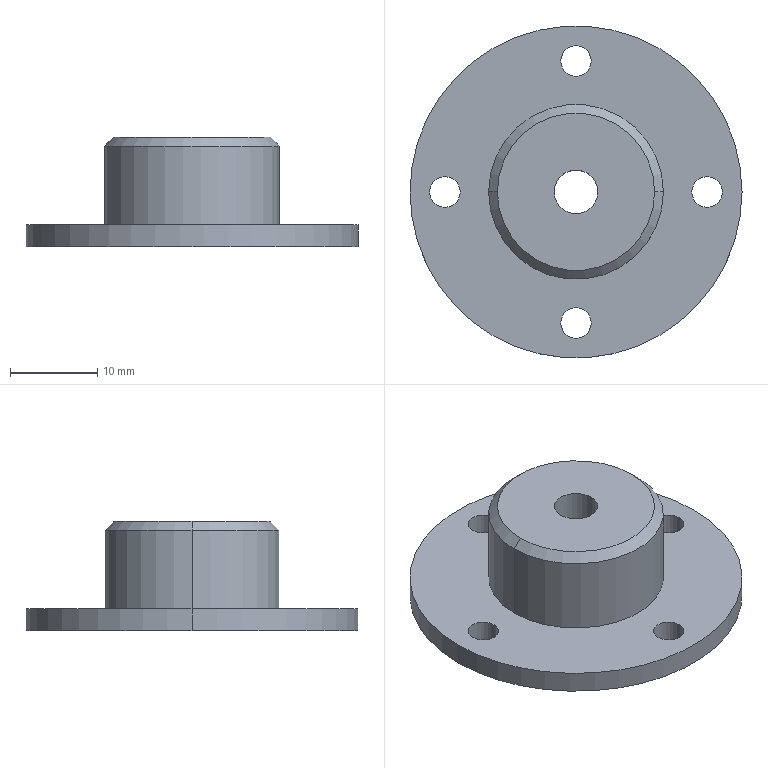Part | SolidWorks | features ICE 2, Chamfer 1, Extrusion 1, HoleWzd 1 | 1 solid | 22 faces | box 38 x 38 x 12.5 mm | volume 5119 mm3 | cylinder 16 | plane 4 | cone 2 | commonest cylinder face diameters 3.5 x8 5 x2 16.5 x2 20 x2 38 x2
STEP:
#1=CARTESIAN_POINT('',(-2.5,0.,2.5));
#2=VERTEX_POINT('',#1);
#3=CARTESIAN_POINT('',(2.5,0.,2.5));
#4=VERTEX_POINT('',#3);
#5=CARTESIAN_POINT('',(0.,0.,2.5));
#6=DIRECTION('',(0.,0.,1.));
#7=DIRECTION('',(1.,0.,0.));
#8=AXIS2_PLACEMENT_3D('',#5,#6,#7);
#9=CIRCLE('',#8,2.5);
#10=EDGE_CURVE('',#2,#4,#9,.T.);
#11=ORIENTED_EDGE('',*,*,#10,.F.);
#12=CARTESIAN_POINT('',(-2.5,0.,12.5));
#13=VERTEX_POINT('',#12);
#14=CARTESIAN_POINT('',(-2.5,0.,12.5));
#15=DIRECTION('',(0.,0.,1.));
#16=VECTOR('',#15,1000.);
#17=LINE('',#14,#16);
#18=EDGE_CURVE('',#2,#13,#17,.T.);
#19=ORIENTED_EDGE('',*,*,#18,.T.);
#20=CARTESIAN_POINT('',(2.5,0.,12.5));
#21=VERTEX_POINT('',#20);
#22=CARTESIAN_POINT('',(0.,0.,12.5));
#23=DIRECTION('',(0.,0.,1.));
#24=DIRECTION('',(1.,0.,0.));
#25=AXIS2_PLACEMENT_3D('',#22,#23,#24);
#26=CIRCLE('',#25,2.5);
#27=EDGE_CURVE('',#13,#21,#26,.T.);
#28=ORIENTED_EDGE('',*,*,#27,.T.);
#29=CARTESIAN_POINT('',(2.5,0.,12.5));
#30=DIRECTION('',(0.,0.,1.));
#31=VECTOR('',#30,1000.);
#32=LINE('',#29,#31);
#33=EDGE_CURVE('',#4,#21,#32,.T.);
#34=ORIENTED_EDGE('',*,*,#33,.F.);
#35=EDGE_LOOP('',(#11,#19,#28,#34));
#36=FACE_OUTER_BOUND('',#35,.T.);
#37=CARTESIAN_POINT('',(0.,0.,12.5));
#38=DIRECTION('',(0.,0.,1.));
#39=DIRECTION('',(1.,0.,0.));
#40=AXIS2_PLACEMENT_3D('',#37,#38,#39);
#41=CYLINDRICAL_SURFACE('',#40,2.5);
#42=ADVANCED_FACE('',(#36),#41,.F.);
#43=CARTESIAN_POINT('',(9.,0.,12.5));
#44=VERTEX_POINT('',#43);
#45=CARTESIAN_POINT('',(-9.,0.,12.5));
#46=VERTEX_POINT('',#45);
#47=CARTESIAN_POINT('',(0.,0.,12.5));
#48=DIRECTION('',(0.,0.,1.));
#49=DIRECTION('',(1.,0.,0.));
#50=AXIS2_PLACEMENT_3D('',#47,#48,#49);
#51=CIRCLE('',#50,9.);
#52=EDGE_CURVE('',#44,#46,#51,.T.);
#53=ORIENTED_EDGE('',*,*,#52,.F.);
#54=CARTESIAN_POINT('',(10.,0.,11.5));
#55=VERTEX_POINT('',#54);
#56=CARTESIAN_POINT('',(9.,0.,12.5));
#57=DIRECTION('',(0.7071,0.,-0.7071));
#58=VECTOR('',#57,1000.);
#59=LINE('',#56,#58);
#60=EDGE_CURVE('',#44,#55,#59,.T.);
#61=ORIENTED_EDGE('',*,*,#60,.T.);
#62=CARTESIAN_POINT('',(-10.,0.,11.5));
#63=VERTEX_POINT('',#62);
#64=CARTESIAN_POINT('',(0.,0.,11.5));
#65=DIRECTION('',(0.,0.,-1.));
#66=DIRECTION('',(1.,0.,0.));
#67=AXIS2_PLACEMENT_3D('',#64,#65,#66);
#68=CIRCLE('',#67,10.);
#69=EDGE_CURVE('',#63,#55,#68,.T.);
#70=ORIENTED_EDGE('',*,*,#69,.F.);
#71=CARTESIAN_POINT('',(-9.,0.,12.5));
#72=DIRECTION('',(-0.7071,0.,-0.7071));
#73=VECTOR('',#72,1000.);
#74=LINE('',#71,#73);
#75=EDGE_CURVE('',#46,#63,#74,.T.);
#76=ORIENTED_EDGE('',*,*,#75,.F.);
#77=EDGE_LOOP('',(#53,#61,#70,#76));
#78=FACE_OUTER_BOUND('',#77,.T.);
#79=CARTESIAN_POINT('',(0.,0.,12.5));
#80=DIRECTION('',(0.,0.,-1.));
#81=DIRECTION('',(-1.,0.,0.));
#82=AXIS2_PLACEMENT_3D('',#79,#80,#81);
#83=CONICAL_SURFACE('',#82,9.,0.7854);
#84=ADVANCED_FACE('',(#78),#83,.T.);
#85=CARTESIAN_POINT('',(-1.75,-15.,0.));
#86=VERTEX_POINT('',#85);
#87=CARTESIAN_POINT('',(1.75,-15.,0.));
#88=VERTEX_POINT('',#87);
#89=CARTESIAN_POINT('',(0.,-15.,0.));
#90=DIRECTION('',(0.,0.,1.));
#91=DIRECTION('',(1.,0.,0.));
#92=AXIS2_PLACEMENT_3D('',#89,#90,#91);
#93=CIRCLE('',#92,1.75);
#94=EDGE_CURVE('',#86,#88,#93,.T.);
#95=ORIENTED_EDGE('',*,*,#94,.F.);
#96=CARTESIAN_POINT('',(-1.75,-15.,2.5));
#97=VERTEX_POINT('',#96);
#98=CARTESIAN_POINT('',(-1.75,-15.,-7.5));
#99=DIRECTION('',(0.,0.,1.));
#100=VECTOR('',#99,1000.);
#101=LINE('',#98,#100);
#102=EDGE_CURVE('',#86,#97,#101,.T.);
#103=ORIENTED_EDGE('',*,*,#102,.T.);
#104=CARTESIAN_POINT('',(1.75,-15.,2.5));
#105=VERTEX_POINT('',#104);
#106=CARTESIAN_POINT('',(0.,-15.,2.5));
#107=DIRECTION('',(0.,0.,1.));
#108=DIRECTION('',(1.,0.,0.));
#109=AXIS2_PLACEMENT_3D('',#106,#107,#108);
#110=CIRCLE('',#109,1.75);
#111=EDGE_CURVE('',#97,#105,#110,.T.);
#112=ORIENTED_EDGE('',*,*,#111,.T.);
#113=CARTESIAN_POINT('',(1.75,-15.,-7.5));
#114=DIRECTION('',(0.,0.,1.));
#115=VECTOR('',#114,1000.);
#116=LINE('',#113,#115);
#117=EDGE_CURVE('',#88,#105,#116,.T.);
#118=ORIENTED_EDGE('',*,*,#117,.F.);
#119=EDGE_LOOP('',(#95,#103,#112,#118));
#120=FACE_OUTER_BOUND('',#119,.T.);
#121=CARTESIAN_POINT('',(0.,-15.,-7.5));
#122=DIRECTION('',(0.,0.,1.));
#123=DIRECTION('',(1.,0.,0.));
#124=AXIS2_PLACEMENT_3D('',#121,#122,#123);
#125=CYLINDRICAL_SURFACE('',#124,1.75);
#126=ADVANCED_FACE('',(#120),#125,.F.);
#127=CARTESIAN_POINT('',(-16.75,0.,0.));
#128=VERTEX_POINT('',#127);
#129=CARTESIAN_POINT('',(-13.25,0.,0.));
#130=VERTEX_POINT('',#129);
#131=CARTESIAN_POINT('',(-15.,0.,0.));
#132=DIRECTION('',(0.,0.,1.));
#133=DIRECTION('',(1.,0.,0.));
#134=AXIS2_PLACEMENT_3D('',#131,#132,#133);
#135=CIRCLE('',#134,1.75);
#136=EDGE_CURVE('',#128,#130,#135,.T.);
#137=ORIENTED_EDGE('',*,*,#136,.F.);
#138=CARTESIAN_POINT('',(-16.75,0.,2.5));
#139=VERTEX_POINT('',#138);
#140=CARTESIAN_POINT('',(-16.75,0.,-7.5));
#141=DIRECTION('',(0.,0.,1.));
#142=VECTOR('',#141,1000.);
#143=LINE('',#140,#142);
#144=EDGE_CURVE('',#128,#139,#143,.T.);
#145=ORIENTED_EDGE('',*,*,#144,.T.);
#146=CARTESIAN_POINT('',(-13.25,0.,2.5));
#147=VERTEX_POINT('',#146);
#148=CARTESIAN_POINT('',(-15.,0.,2.5));
#149=DIRECTION('',(0.,0.,1.));
#150=DIRECTION('',(1.,0.,0.));
#151=AXIS2_PLACEMENT_3D('',#148,#149,#150);
#152=CIRCLE('',#151,1.75);
#153=EDGE_CURVE('',#139,#147,#152,.T.);
#154=ORIENTED_EDGE('',*,*,#153,.T.);
#155=CARTESIAN_POINT('',(-13.25,0.,-7.5));
#156=DIRECTION('',(0.,0.,1.));
#157=VECTOR('',#156,1000.);
#158=LINE('',#155,#157);
#159=EDGE_CURVE('',#130,#147,#158,.T.);
#160=ORIENTED_EDGE('',*,*,#159,.F.);
#161=EDGE_LOOP('',(#137,#145,#154,#160));
#162=FACE_OUTER_BOUND('',#161,.T.);
#163=CARTESIAN_POINT('',(-15.,0.,-7.5));
#164=DIRECTION('',(0.,0.,1.));
#165=DIRECTION('',(1.,0.,0.));
#166=AXIS2_PLACEMENT_3D('',#163,#164,#165);
#167=CYLINDRICAL_SURFACE('',#166,1.75);
#168=ADVANCED_FACE('',(#162),#167,.F.);
#169=CARTESIAN_POINT('',(-1.75,15.,0.));
#170=VERTEX_POINT('',#169);
#171=CARTESIAN_POINT('',(1.75,15.,0.));
#172=VERTEX_POINT('',#171);
#173=CARTESIAN_POINT('',(0.,15.,0.));
#174=DIRECTION('',(0.,0.,1.));
#175=DIRECTION('',(1.,0.,0.));
#176=AXIS2_PLACEMENT_3D('',#173,#174,#175);
#177=CIRCLE('',#176,1.75);
#178=EDGE_CURVE('',#170,#172,#177,.T.);
#179=ORIENTED_EDGE('',*,*,#178,.F.);
#180=CARTESIAN_POINT('',(-1.75,15.,2.5));
#181=VERTEX_POINT('',#180);
#182=CARTESIAN_POINT('',(-1.75,15.,-7.5));
#183=DIRECTION('',(0.,0.,1.));
#184=VECTOR('',#183,1000.);
#185=LINE('',#182,#184);
#186=EDGE_CURVE('',#170,#181,#185,.T.);
#187=ORIENTED_EDGE('',*,*,#186,.T.);
#188=CARTESIAN_POINT('',(1.75,15.,2.5));
#189=VERTEX_POINT('',#188);
#190=CARTESIAN_POINT('',(0.,15.,2.5));
#191=DIRECTION('',(0.,0.,1.));
#192=DIRECTION('',(1.,0.,0.));
#193=AXIS2_PLACEMENT_3D('',#190,#191,#192);
#194=CIRCLE('',#193,1.75);
#195=EDGE_CURVE('',#181,#189,#194,.T.);
#196=ORIENTED_EDGE('',*,*,#195,.T.);
#197=CARTESIAN_POINT('',(1.75,15.,-7.5));
#198=DIRECTION('',(0.,0.,1.));
#199=VECTOR('',#198,1000.);
#200=LINE('',#197,#199);
#201=EDGE_CURVE('',#172,#189,#200,.T.);
#202=ORIENTED_EDGE('',*,*,#201,.F.);
#203=EDGE_LOOP('',(#179,#187,#196,#202));
#204=FACE_OUTER_BOUND('',#203,.T.);
#205=CARTESIAN_POINT('',(0.,15.,-7.5));
#206=DIRECTION('',(0.,0.,1.));
#207=DIRECTION('',(1.,0.,0.));
#208=AXIS2_PLACEMENT_3D('',#205,#206,#207);
#209=CYLINDRICAL_SURFACE('',#208,1.75);
#210=ADVANCED_FACE('',(#204),#209,.F.);
#211=CARTESIAN_POINT('',(13.25,0.,0.));
#212=VERTEX_POINT('',#211);
#213=CARTESIAN_POINT('',(16.75,0.,0.));
#214=VERTEX_POINT('',#213);
#215=CARTESIAN_POINT('',(15.,0.,0.));
#216=DIRECTION('',(0.,0.,1.));
#217=DIRECTION('',(1.,0.,0.));
#218=AXIS2_PLACEMENT_3D('',#215,#216,#217);
#219=CIRCLE('',#218,1.75);
#220=EDGE_CURVE('',#212,#214,#219,.T.);
#221=ORIENTED_EDGE('',*,*,#220,.F.);
#222=CARTESIAN_POINT('',(13.25,0.,2.5));
#223=VERTEX_POINT('',#222);
#224=CARTESIAN_POINT('',(13.25,0.,-7.5));
#225=DIRECTION('',(0.,0.,1.));
#226=VECTOR('',#225,1000.);
#227=LINE('',#224,#226);
#228=EDGE_CURVE('',#212,#223,#227,.T.);
#229=ORIENTED_EDGE('',*,*,#228,.T.);
#230=CARTESIAN_POINT('',(16.75,0.,2.5));
#231=VERTEX_POINT('',#230);
#232=CARTESIAN_POINT('',(15.,0.,2.5));
#233=DIRECTION('',(0.,0.,1.));
#234=DIRECTION('',(1.,0.,0.));
#235=AXIS2_PLACEMENT_3D('',#232,#233,#234);
#236=CIRCLE('',#235,1.75);
#237=EDGE_CURVE('',#223,#231,#236,.T.);
#238=ORIENTED_EDGE('',*,*,#237,.T.);
#239=CARTESIAN_POINT('',(16.75,0.,-7.5));
#240=DIRECTION('',(0.,0.,1.));
#241=VECTOR('',#240,1000.);
#242=LINE('',#239,#241);
#243=EDGE_CURVE('',#214,#231,#242,.T.);
#244=ORIENTED_EDGE('',*,*,#243,.F.);
#245=EDGE_LOOP('',(#221,#229,#238,#244));
#246=FACE_OUTER_BOUND('',#245,.T.);
#247=CARTESIAN_POINT('',(15.,0.,-7.5));
#248=DIRECTION('',(0.,0.,1.));
#249=DIRECTION('',(1.,0.,0.));
#250=AXIS2_PLACEMENT_3D('',#247,#248,#249);
#251=CYLINDRICAL_SURFACE('',#250,1.75);
#252=ADVANCED_FACE('',(#246),#251,.F.);
#253=ORIENTED_EDGE('',*,*,#69,.T.);
#254=CARTESIAN_POINT('',(10.,0.,2.5));
#255=VERTEX_POINT('',#254);
#256=CARTESIAN_POINT('',(10.,0.,12.5));
#257=DIRECTION('',(0.,0.,-1.));
#258=VECTOR('',#257,1000.);
#259=LINE('',#256,#258);
#260=EDGE_CURVE('',#55,#255,#259,.T.);
#261=ORIENTED_EDGE('',*,*,#260,.T.);
#262=CARTESIAN_POINT('',(-10.,0.,2.5));
#263=VERTEX_POINT('',#262);
#264=CARTESIAN_POINT('',(0.,0.,2.5));
#265=DIRECTION('',(0.,0.,1.));
#266=DIRECTION('',(1.,0.,0.));
#267=AXIS2_PLACEMENT_3D('',#264,#265,#266);
#268=CIRCLE('',#267,10.);
#269=EDGE_CURVE('',#255,#263,#268,.T.);
#270=ORIENTED_EDGE('',*,*,#269,.T.);
#271=CARTESIAN_POINT('',(-10.,0.,12.5));
#272=DIRECTION('',(0.,0.,-1.));
#273=VECTOR('',#272,1000.);
#274=LINE('',#271,#273);
#275=EDGE_CURVE('',#63,#263,#274,.T.);
#276=ORIENTED_EDGE('',*,*,#275,.F.);
#277=EDGE_LOOP('',(#253,#261,#270,#276));
#278=FACE_OUTER_BOUND('',#277,.T.);
#279=CARTESIAN_POINT('',(0.,0.,12.5));
#280=DIRECTION('',(0.,0.,-1.));
#281=DIRECTION('',(-1.,0.,0.));
#282=AXIS2_PLACEMENT_3D('',#279,#280,#281);
#283=CYLINDRICAL_SURFACE('',#282,10.);
#284=ADVANCED_FACE('',(#278),#283,.T.);
#285=CARTESIAN_POINT('',(-8.25,0.,2.5));
#286=VERTEX_POINT('',#285);
#287=CARTESIAN_POINT('',(8.25,0.,2.5));
#288=VERTEX_POINT('',#287);
#289=CARTESIAN_POINT('',(0.,0.,2.5));
#290=DIRECTION('',(0.,0.,1.));
#291=DIRECTION('',(1.,0.,0.));
#292=AXIS2_PLACEMENT_3D('',#289,#290,#291);
#293=CIRCLE('',#292,8.25);
#294=EDGE_CURVE('',#286,#288,#293,.T.);
#295=ORIENTED_EDGE('',*,*,#294,.T.);
#296=CARTESIAN_POINT('',(8.25,0.,0.));
#297=VERTEX_POINT('',#296);
#298=CARTESIAN_POINT('',(8.25,0.,2.5));
#299=DIRECTION('',(0.,0.,-1.));
#300=VECTOR('',#299,1000.);
#301=LINE('',#298,#300);
#302=EDGE_CURVE('',#288,#297,#301,.T.);
#303=ORIENTED_EDGE('',*,*,#302,.T.);
#304=CARTESIAN_POINT('',(-8.25,0.,0.));
#305=VERTEX_POINT('',#304);
#306=CARTESIAN_POINT('',(0.,0.,0.));
#307=DIRECTION('',(0.,0.,1.));
#308=DIRECTION('',(1.,0.,0.));
#309=AXIS2_PLACEMENT_3D('',#306,#307,#308);
#310=CIRCLE('',#309,8.25);
#311=EDGE_CURVE('',#305,#297,#310,.T.);
#312=ORIENTED_EDGE('',*,*,#311,.F.);
#313=CARTESIAN_POINT('',(-8.25,0.,2.5));
#314=DIRECTION('',(0.,0.,-1.));
#315=VECTOR('',#314,1000.);
#316=LINE('',#313,#315);
#317=EDGE_CURVE('',#286,#305,#316,.T.);
#318=ORIENTED_EDGE('',*,*,#317,.F.);
#319=EDGE_LOOP('',(#295,#303,#312,#318));
#320=FACE_OUTER_BOUND('',#319,.T.);
#321=CARTESIAN_POINT('',(0.,0.,2.5));
#322=DIRECTION('',(0.,0.,-1.));
#323=DIRECTION('',(-1.,0.,0.));
#324=AXIS2_PLACEMENT_3D('',#321,#322,#323);
#325=CYLINDRICAL_SURFACE('',#324,8.25);
#326=ADVANCED_FACE('',(#320),#325,.F.);
#327=CARTESIAN_POINT('',(19.,0.,2.5));
#328=VERTEX_POINT('',#327);
#329=CARTESIAN_POINT('',(-19.,0.,2.5));
#330=VERTEX_POINT('',#329);
#331=CARTESIAN_POINT('',(0.,0.,2.5));
#332=DIRECTION('',(0.,0.,1.));
#333=DIRECTION('',(1.,0.,0.));
#334=AXIS2_PLACEMENT_3D('',#331,#332,#333);
#335=CIRCLE('',#334,19.);
#336=EDGE_CURVE('',#328,#330,#335,.T.);
#337=ORIENTED_EDGE('',*,*,#336,.F.);
#338=CARTESIAN_POINT('',(19.,0.,0.));
#339=VERTEX_POINT('',#338);
#340=CARTESIAN_POINT('',(19.,0.,2.5));
#341=DIRECTION('',(0.,0.,-1.));
#342=VECTOR('',#341,1000.);
#343=LINE('',#340,#342);
#344=EDGE_CURVE('',#328,#339,#343,.T.);
#345=ORIENTED_EDGE('',*,*,#344,.T.);
#346=CARTESIAN_POINT('',(-19.,0.,0.));
#347=VERTEX_POINT('',#346);
#348=CARTESIAN_POINT('',(0.,0.,0.));
#349=DIRECTION('',(0.,0.,1.));
#350=DIRECTION('',(1.,0.,0.));
#351=AXIS2_PLACEMENT_3D('',#348,#349,#350);
#352=CIRCLE('',#351,19.);
#353=EDGE_CURVE('',#339,#347,#352,.T.);
#354=ORIENTED_EDGE('',*,*,#353,.T.);
#355=CARTESIAN_POINT('',(-19.,0.,2.5));
#356=DIRECTION('',(0.,0.,-1.));
#357=VECTOR('',#356,1000.);
#358=LINE('',#355,#357);
#359=EDGE_CURVE('',#330,#347,#358,.T.);
#360=ORIENTED_EDGE('',*,*,#359,.F.);
#361=EDGE_LOOP('',(#337,#345,#354,#360));
#362=FACE_OUTER_BOUND('',#361,.T.);
#363=CARTESIAN_POINT('',(0.,0.,2.5));
#364=DIRECTION('',(0.,0.,-1.));
#365=DIRECTION('',(-1.,0.,0.));
#366=AXIS2_PLACEMENT_3D('',#363,#364,#365);
#367=CYLINDRICAL_SURFACE('',#366,19.);
#368=ADVANCED_FACE('',(#362),#367,.T.);
#369=CARTESIAN_POINT('',(0.,-15.,2.5));
#370=DIRECTION('',(0.,0.,1.));
#371=DIRECTION('',(1.,0.,0.));
#372=AXIS2_PLACEMENT_3D('',#369,#370,#371);
#373=CIRCLE('',#372,1.75);
#374=EDGE_CURVE('',#105,#97,#373,.T.);
#375=ORIENTED_EDGE('',*,*,#374,.F.);
#376=ORIENTED_EDGE('',*,*,#111,.F.);
#377=EDGE_LOOP('',(#375,#376));
#378=FACE_BOUND('',#377,.T.);
#379=CARTESIAN_POINT('',(-15.,0.,2.5));
#380=DIRECTION('',(0.,0.,1.));
#381=DIRECTION('',(1.,0.,0.));
#382=AXIS2_PLACEMENT_3D('',#379,#380,#381);
#383=CIRCLE('',#382,1.75);
#384=EDGE_CURVE('',#147,#139,#383,.T.);
#385=ORIENTED_EDGE('',*,*,#384,.F.);
#386=ORIENTED_EDGE('',*,*,#153,.F.);
#387=EDGE_LOOP('',(#385,#386));
#388=FACE_BOUND('',#387,.T.);
#389=CARTESIAN_POINT('',(0.,15.,2.5));
#390=DIRECTION('',(0.,0.,1.));
#391=DIRECTION('',(1.,0.,0.));
#392=AXIS2_PLACEMENT_3D('',#389,#390,#391);
#393=CIRCLE('',#392,1.75);
#394=EDGE_CURVE('',#189,#181,#393,.T.);
#395=ORIENTED_EDGE('',*,*,#394,.F.);
#396=ORIENTED_EDGE('',*,*,#195,.F.);
#397=EDGE_LOOP('',(#395,#396));
#398=FACE_BOUND('',#397,.T.);
#399=CARTESIAN_POINT('',(15.,0.,2.5));
#400=DIRECTION('',(0.,0.,1.));
#401=DIRECTION('',(1.,0.,0.));
#402=AXIS2_PLACEMENT_3D('',#399,#400,#401);
#403=CIRCLE('',#402,1.75);
#404=EDGE_CURVE('',#231,#223,#403,.T.);
#405=ORIENTED_EDGE('',*,*,#404,.F.);
#406=ORIENTED_EDGE('',*,*,#237,.F.);
#407=EDGE_LOOP('',(#405,#406));
#408=FACE_BOUND('',#407,.T.);
#409=CARTESIAN_POINT('',(0.,0.,2.5));
#410=DIRECTION('',(0.,0.,1.));
#411=DIRECTION('',(1.,0.,0.));
#412=AXIS2_PLACEMENT_3D('',#409,#410,#411);
#413=CIRCLE('',#412,19.);
#414=EDGE_CURVE('',#330,#328,#413,.T.);
#415=ORIENTED_EDGE('',*,*,#414,.T.);
#416=ORIENTED_EDGE('',*,*,#336,.T.);
#417=EDGE_LOOP('',(#415,#416));
#418=FACE_OUTER_BOUND('',#417,.T.);
#419=CARTESIAN_POINT('',(0.,0.,2.5));
#420=DIRECTION('',(0.,0.,1.));
#421=DIRECTION('',(1.,0.,0.));
#422=AXIS2_PLACEMENT_3D('',#419,#420,#421);
#423=CIRCLE('',#422,10.);
#424=EDGE_CURVE('',#263,#255,#423,.T.);
#425=ORIENTED_EDGE('',*,*,#424,.F.);
#426=ORIENTED_EDGE('',*,*,#269,.F.);
#427=EDGE_LOOP('',(#425,#426));
#428=FACE_BOUND('',#427,.T.);
#429=CARTESIAN_POINT('',(0.,0.,2.5));
#430=DIRECTION('',(0.,0.,1.));
#431=DIRECTION('',(1.,0.,0.));
#432=AXIS2_PLACEMENT_3D('',#429,#430,#431);
#433=PLANE('',#432);
#434=ADVANCED_FACE('',(#378,#388,#398,#408,#418,#428),#433,.T.);
#435=CARTESIAN_POINT('',(0.,-15.,0.));
#436=DIRECTION('',(0.,0.,1.));
#437=DIRECTION('',(1.,0.,0.));
#438=AXIS2_PLACEMENT_3D('',#435,#436,#437);
#439=CIRCLE('',#438,1.75);
#440=EDGE_CURVE('',#88,#86,#439,.T.);
#441=ORIENTED_EDGE('',*,*,#440,.T.);
#442=ORIENTED_EDGE('',*,*,#94,.T.);
#443=EDGE_LOOP('',(#441,#442));
#444=FACE_BOUND('',#443,.T.);
#445=CARTESIAN_POINT('',(-15.,0.,0.));
#446=DIRECTION('',(0.,0.,1.));
#447=DIRECTION('',(1.,0.,0.));
#448=AXIS2_PLACEMENT_3D('',#445,#446,#447);
#449=CIRCLE('',#448,1.75);
#450=EDGE_CURVE('',#130,#128,#449,.T.);
#451=ORIENTED_EDGE('',*,*,#450,.T.);
#452=ORIENTED_EDGE('',*,*,#136,.T.);
#453=EDGE_LOOP('',(#451,#452));
#454=FACE_BOUND('',#453,.T.);
#455=CARTESIAN_POINT('',(0.,15.,0.));
#456=DIRECTION('',(0.,0.,1.));
#457=DIRECTION('',(1.,0.,0.));
#458=AXIS2_PLACEMENT_3D('',#455,#456,#457);
#459=CIRCLE('',#458,1.75);
#460=EDGE_CURVE('',#172,#170,#459,.T.);
#461=ORIENTED_EDGE('',*,*,#460,.T.);
#462=ORIENTED_EDGE('',*,*,#178,.T.);
#463=EDGE_LOOP('',(#461,#462));
#464=FACE_BOUND('',#463,.T.);
#465=CARTESIAN_POINT('',(15.,0.,0.));
#466=DIRECTION('',(0.,0.,1.));
#467=DIRECTION('',(1.,0.,0.));
#468=AXIS2_PLACEMENT_3D('',#465,#466,#467);
#469=CIRCLE('',#468,1.75);
#470=EDGE_CURVE('',#214,#212,#469,.T.);
#471=ORIENTED_EDGE('',*,*,#470,.T.);
#472=ORIENTED_EDGE('',*,*,#220,.T.);
#473=EDGE_LOOP('',(#471,#472));
#474=FACE_BOUND('',#473,.T.);
#475=CARTESIAN_POINT('',(0.,0.,0.));
#476=DIRECTION('',(0.,0.,1.));
#477=DIRECTION('',(1.,0.,0.));
#478=AXIS2_PLACEMENT_3D('',#475,#476,#477);
#479=CIRCLE('',#478,19.);
#480=EDGE_CURVE('',#347,#339,#479,.T.);
#481=ORIENTED_EDGE('',*,*,#480,.F.);
#482=ORIENTED_EDGE('',*,*,#353,.F.);
#483=EDGE_LOOP('',(#481,#482));
#484=FACE_OUTER_BOUND('',#483,.T.);
#485=ORIENTED_EDGE('',*,*,#311,.T.);
#486=CARTESIAN_POINT('',(0.,0.,0.));
#487=DIRECTION('',(0.,0.,1.));
#488=DIRECTION('',(1.,0.,0.));
#489=AXIS2_PLACEMENT_3D('',#486,#487,#488);
#490=CIRCLE('',#489,8.25);
#491=EDGE_CURVE('',#297,#305,#490,.T.);
#492=ORIENTED_EDGE('',*,*,#491,.T.);
#493=EDGE_LOOP('',(#485,#492));
#494=FACE_BOUND('',#493,.T.);
#495=CARTESIAN_POINT('',(0.,0.,0.));
#496=DIRECTION('',(0.,0.,1.));
#497=DIRECTION('',(1.,0.,0.));
#498=AXIS2_PLACEMENT_3D('',#495,#496,#497);
#499=PLANE('',#498);
#500=ADVANCED_FACE('',(#444,#454,#464,#474,#484,#494),#499,.F.);
#501=ORIENTED_EDGE('',*,*,#344,.F.);
#502=ORIENTED_EDGE('',*,*,#414,.F.);
#503=ORIENTED_EDGE('',*,*,#359,.T.);
#504=ORIENTED_EDGE('',*,*,#480,.T.);
#505=EDGE_LOOP('',(#501,#502,#503,#504));
#506=FACE_OUTER_BOUND('',#505,.T.);
#507=CARTESIAN_POINT('',(0.,0.,2.5));
#508=DIRECTION('',(0.,0.,-1.));
#509=DIRECTION('',(-1.,0.,0.));
#510=AXIS2_PLACEMENT_3D('',#507,#508,#509);
#511=CYLINDRICAL_SURFACE('',#510,19.);
#512=ADVANCED_FACE('',(#506),#511,.T.);
#513=ORIENTED_EDGE('',*,*,#302,.F.);
#514=CARTESIAN_POINT('',(0.,0.,2.5));
#515=DIRECTION('',(0.,0.,1.));
#516=DIRECTION('',(1.,0.,0.));
#517=AXIS2_PLACEMENT_3D('',#514,#515,#516);
#518=CIRCLE('',#517,8.25);
#519=EDGE_CURVE('',#288,#286,#518,.T.);
#520=ORIENTED_EDGE('',*,*,#519,.T.);
#521=ORIENTED_EDGE('',*,*,#317,.T.);
#522=ORIENTED_EDGE('',*,*,#491,.F.);
#523=EDGE_LOOP('',(#513,#520,#521,#522));
#524=FACE_OUTER_BOUND('',#523,.T.);
#525=CARTESIAN_POINT('',(0.,0.,2.5));
#526=DIRECTION('',(0.,0.,-1.));
#527=DIRECTION('',(-1.,0.,0.));
#528=AXIS2_PLACEMENT_3D('',#525,#526,#527);
#529=CYLINDRICAL_SURFACE('',#528,8.25);
#530=ADVANCED_FACE('',(#524),#529,.F.);
#531=CARTESIAN_POINT('',(0.,0.,2.5));
#532=DIRECTION('',(0.,0.,1.));
#533=DIRECTION('',(1.,0.,0.));
#534=AXIS2_PLACEMENT_3D('',#531,#532,#533);
#535=CIRCLE('',#534,2.5);
#536=EDGE_CURVE('',#4,#2,#535,.T.);
#537=ORIENTED_EDGE('',*,*,#536,.T.);
#538=ORIENTED_EDGE('',*,*,#10,.T.);
#539=EDGE_LOOP('',(#537,#538));
#540=FACE_BOUND('',#539,.T.);
#541=ORIENTED_EDGE('',*,*,#294,.F.);
#542=ORIENTED_EDGE('',*,*,#519,.F.);
#543=EDGE_LOOP('',(#541,#542));
#544=FACE_OUTER_BOUND('',#543,.T.);
#545=CARTESIAN_POINT('',(0.,0.,2.5));
#546=DIRECTION('',(0.,0.,1.));
#547=DIRECTION('',(1.,0.,0.));
#548=AXIS2_PLACEMENT_3D('',#545,#546,#547);
#549=PLANE('',#548);
#550=ADVANCED_FACE('',(#540,#544),#549,.F.);
#551=ORIENTED_EDGE('',*,*,#260,.F.);
#552=CARTESIAN_POINT('',(0.,0.,11.5));
#553=DIRECTION('',(0.,0.,-1.));
#554=DIRECTION('',(1.,0.,0.));
#555=AXIS2_PLACEMENT_3D('',#552,#553,#554);
#556=CIRCLE('',#555,10.);
#557=EDGE_CURVE('',#55,#63,#556,.T.);
#558=ORIENTED_EDGE('',*,*,#557,.T.);
#559=ORIENTED_EDGE('',*,*,#275,.T.);
#560=ORIENTED_EDGE('',*,*,#424,.T.);
#561=EDGE_LOOP('',(#551,#558,#559,#560));
#562=FACE_OUTER_BOUND('',#561,.T.);
#563=CARTESIAN_POINT('',(0.,0.,12.5));
#564=DIRECTION('',(0.,0.,-1.));
#565=DIRECTION('',(-1.,0.,0.));
#566=AXIS2_PLACEMENT_3D('',#563,#564,#565);
#567=CYLINDRICAL_SURFACE('',#566,10.);
#568=ADVANCED_FACE('',(#562),#567,.T.);
#569=CARTESIAN_POINT('',(0.,0.,12.5));
#570=DIRECTION('',(0.,0.,1.));
#571=DIRECTION('',(1.,0.,0.));
#572=AXIS2_PLACEMENT_3D('',#569,#570,#571);
#573=CIRCLE('',#572,2.5);
#574=EDGE_CURVE('',#21,#13,#573,.T.);
#575=ORIENTED_EDGE('',*,*,#574,.F.);
#576=ORIENTED_EDGE('',*,*,#27,.F.);
#577=EDGE_LOOP('',(#575,#576));
#578=FACE_BOUND('',#577,.T.);
#579=CARTESIAN_POINT('',(0.,0.,12.5));
#580=DIRECTION('',(0.,0.,1.));
#581=DIRECTION('',(1.,0.,0.));
#582=AXIS2_PLACEMENT_3D('',#579,#580,#581);
#583=CIRCLE('',#582,9.);
#584=EDGE_CURVE('',#46,#44,#583,.T.);
#585=ORIENTED_EDGE('',*,*,#584,.T.);
#586=ORIENTED_EDGE('',*,*,#52,.T.);
#587=EDGE_LOOP('',(#585,#586));
#588=FACE_OUTER_BOUND('',#587,.T.);
#589=CARTESIAN_POINT('',(0.,0.,12.5));
#590=DIRECTION('',(0.,0.,1.));
#591=DIRECTION('',(1.,0.,0.));
#592=AXIS2_PLACEMENT_3D('',#589,#590,#591);
#593=PLANE('',#592);
#594=ADVANCED_FACE('',(#578,#588),#593,.T.);
#595=ORIENTED_EDGE('',*,*,#228,.F.);
#596=ORIENTED_EDGE('',*,*,#470,.F.);
#597=ORIENTED_EDGE('',*,*,#243,.T.);
#598=ORIENTED_EDGE('',*,*,#404,.T.);
#599=EDGE_LOOP('',(#595,#596,#597,#598));
#600=FACE_OUTER_BOUND('',#599,.T.);
#601=CARTESIAN_POINT('',(15.,0.,-7.5));
#602=DIRECTION('',(0.,0.,1.));
#603=DIRECTION('',(1.,0.,0.));
#604=AXIS2_PLACEMENT_3D('',#601,#602,#603);
#605=CYLINDRICAL_SURFACE('',#604,1.75);
#606=ADVANCED_FACE('',(#600),#605,.F.);
#607=ORIENTED_EDGE('',*,*,#186,.F.);
#608=ORIENTED_EDGE('',*,*,#460,.F.);
#609=ORIENTED_EDGE('',*,*,#201,.T.);
#610=ORIENTED_EDGE('',*,*,#394,.T.);
#611=EDGE_LOOP('',(#607,#608,#609,#610));
#612=FACE_OUTER_BOUND('',#611,.T.);
#613=CARTESIAN_POINT('',(0.,15.,-7.5));
#614=DIRECTION('',(0.,0.,1.));
#615=DIRECTION('',(1.,0.,0.));
#616=AXIS2_PLACEMENT_3D('',#613,#614,#615);
#617=CYLINDRICAL_SURFACE('',#616,1.75);
#618=ADVANCED_FACE('',(#612),#617,.F.);
#619=ORIENTED_EDGE('',*,*,#144,.F.);
#620=ORIENTED_EDGE('',*,*,#450,.F.);
#621=ORIENTED_EDGE('',*,*,#159,.T.);
#622=ORIENTED_EDGE('',*,*,#384,.T.);
#623=EDGE_LOOP('',(#619,#620,#621,#622));
#624=FACE_OUTER_BOUND('',#623,.T.);
#625=CARTESIAN_POINT('',(-15.,0.,-7.5));
#626=DIRECTION('',(0.,0.,1.));
#627=DIRECTION('',(1.,0.,0.));
#628=AXIS2_PLACEMENT_3D('',#625,#626,#627);
#629=CYLINDRICAL_SURFACE('',#628,1.75);
#630=ADVANCED_FACE('',(#624),#629,.F.);
#631=ORIENTED_EDGE('',*,*,#102,.F.);
#632=ORIENTED_EDGE('',*,*,#440,.F.);
#633=ORIENTED_EDGE('',*,*,#117,.T.);
#634=ORIENTED_EDGE('',*,*,#374,.T.);
#635=EDGE_LOOP('',(#631,#632,#633,#634));
#636=FACE_OUTER_BOUND('',#635,.T.);
#637=CARTESIAN_POINT('',(0.,-15.,-7.5));
#638=DIRECTION('',(0.,0.,1.));
#639=DIRECTION('',(1.,0.,0.));
#640=AXIS2_PLACEMENT_3D('',#637,#638,#639);
#641=CYLINDRICAL_SURFACE('',#640,1.75);
#642=ADVANCED_FACE('',(#636),#641,.F.);
#643=ORIENTED_EDGE('',*,*,#60,.F.);
#644=ORIENTED_EDGE('',*,*,#584,.F.);
#645=ORIENTED_EDGE('',*,*,#75,.T.);
#646=ORIENTED_EDGE('',*,*,#557,.F.);
#647=EDGE_LOOP('',(#643,#644,#645,#646));
#648=FACE_OUTER_BOUND('',#647,.T.);
#649=CARTESIAN_POINT('',(0.,0.,12.5));
#650=DIRECTION('',(0.,0.,-1.));
#651=DIRECTION('',(-1.,0.,0.));
#652=AXIS2_PLACEMENT_3D('',#649,#650,#651);
#653=CONICAL_SURFACE('',#652,9.,0.7854);
#654=ADVANCED_FACE('',(#648),#653,.T.);
#655=ORIENTED_EDGE('',*,*,#18,.F.);
#656=ORIENTED_EDGE('',*,*,#536,.F.);
#657=ORIENTED_EDGE('',*,*,#33,.T.);
#658=ORIENTED_EDGE('',*,*,#574,.T.);
#659=EDGE_LOOP('',(#655,#656,#657,#658));
#660=FACE_OUTER_BOUND('',#659,.T.);
#661=CARTESIAN_POINT('',(0.,0.,12.5));
#662=DIRECTION('',(0.,0.,1.));
#663=DIRECTION('',(1.,0.,0.));
#664=AXIS2_PLACEMENT_3D('',#661,#662,#663);
#665=CYLINDRICAL_SURFACE('',#664,2.5);
#666=ADVANCED_FACE('',(#660),#665,.F.);
#667=CLOSED_SHELL('',(#42,#84,#126,#168,#210,#252,#284,#326,#368,#434,#500,#512,#530,#550,#568,#594,#606,#618,#630,#642,#654,#666));
#668=MANIFOLD_SOLID_BREP('',#667);
#669=CARTESIAN_POINT('',(0.,0.,0.));
#670=DIRECTION('',(0.,0.,1.));
#671=DIRECTION('',(1.,0.,0.));
#672=AXIS2_PLACEMENT_3D('',#669,#670,#671);
#673=(LENGTH_UNIT()NAMED_UNIT(*)SI_UNIT(.MILLI.,.METRE.));
#674=UNCERTAINTY_MEASURE_WITH_UNIT(LENGTH_MEASURE(0.00001),#673,'','');
#675=(NAMED_UNIT(*)PLANE_ANGLE_UNIT()SI_UNIT($,.RADIAN.));
#676=(NAMED_UNIT(*)SI_UNIT($,.STERADIAN.)SOLID_ANGLE_UNIT());
#677=(GEOMETRIC_REPRESENTATION_CONTEXT(3)GLOBAL_UNCERTAINTY_ASSIGNED_CONTEXT((#674))GLOBAL_UNIT_ASSIGNED_CONTEXT((#673,#675,#676))REPRESENTATION_CONTEXT('',''));
#678=ADVANCED_BREP_SHAPE_REPRESENTATION('',(#668,#672),#677);